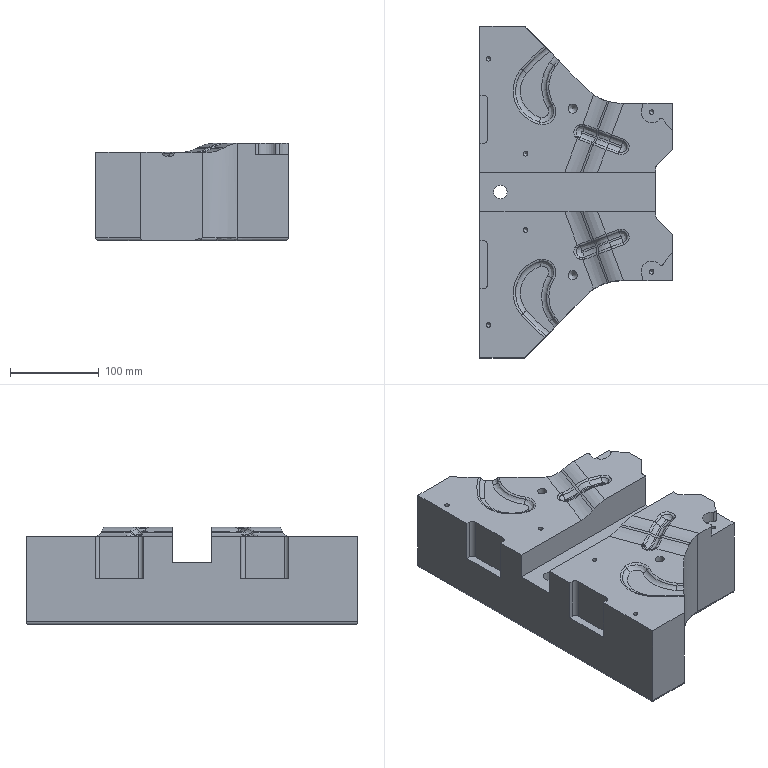Part | NX | features solid 2 | 1 solid | 162 faces | box 217 x 374 x 109.5 mm | volume 5563191 mm3 | cylinder 58 | plane 40 | spline 40 | torus 16 | cone 8 | commonest cylinder face diameters 6 x19 13 x8 5.2 x6 10 x6 63 x4 67 x4